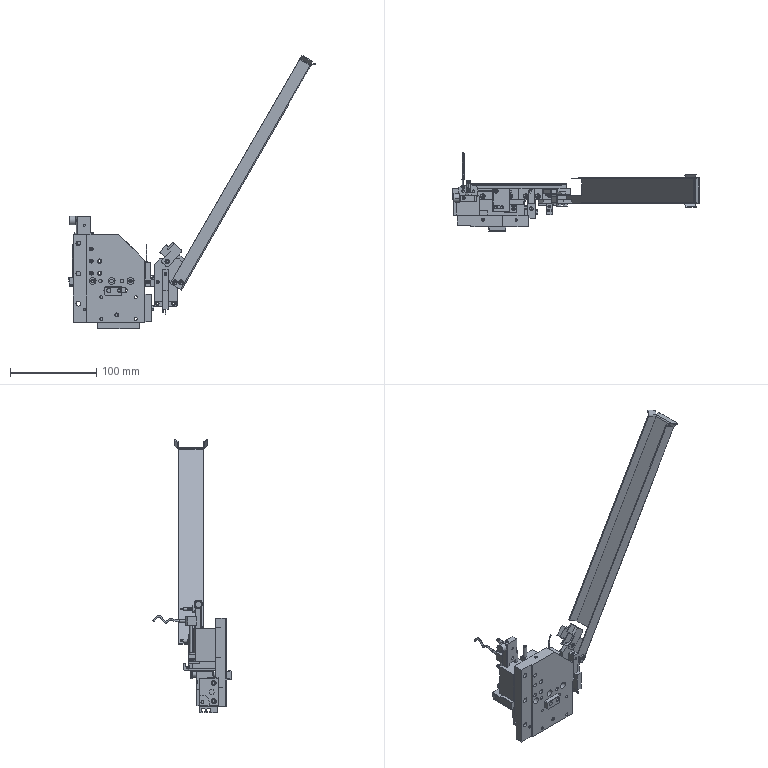Part | NX | 54 solids | 2618 faces | box 285.673 x 90.618 x 317.186 mm | volume 249194 mm3 | plane 1733 | cylinder 596 | cone 257 | spline 18 | torus 13 | sphere 1 | commonest cylinder face diameters 2.5 x99 4 x88 3 x58 3.3 x46 6 x30 5 x28